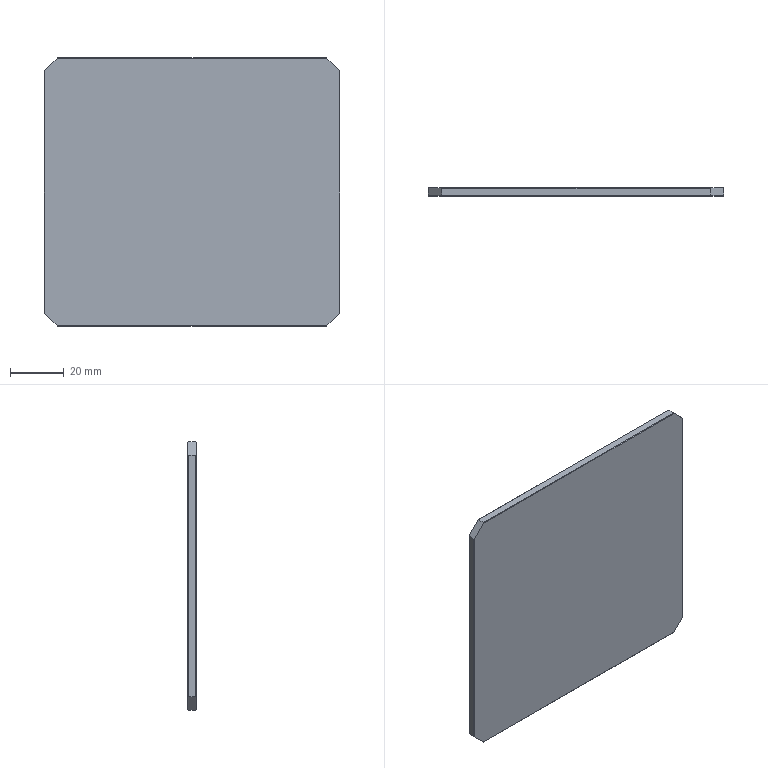Part | SolidWorks | features Chamfer 2, Extrusion 1, HoleWzd 1 | 1 solid | 18 faces | box 110 x 3 x 100 mm | volume 32835 mm3 | plane 18
STEP:
#1=CARTESIAN_POINT('',(-55.,2.8,-45.));
#2=VERTEX_POINT('',#1);
#3=CARTESIAN_POINT('',(-55.,0.2,-45.));
#4=VERTEX_POINT('',#3);
#5=CARTESIAN_POINT('',(-55.,3.,-45.));
#6=DIRECTION('',(0.,-1.,0.));
#7=VECTOR('',#6,1000.);
#8=LINE('',#5,#7);
#9=EDGE_CURVE('',#2,#4,#8,.T.);
#10=ORIENTED_EDGE('',*,*,#9,.T.);
#11=CARTESIAN_POINT('',(-55.,0.2,45.));
#12=VERTEX_POINT('',#11);
#13=CARTESIAN_POINT('',(-55.,0.2,50.));
#14=DIRECTION('',(0.,0.,1.));
#15=VECTOR('',#14,1000.);
#16=LINE('',#13,#15);
#17=EDGE_CURVE('',#4,#12,#16,.T.);
#18=ORIENTED_EDGE('',*,*,#17,.T.);
#19=CARTESIAN_POINT('',(-55.,2.8,45.));
#20=VERTEX_POINT('',#19);
#21=CARTESIAN_POINT('',(-55.,3.,45.));
#22=DIRECTION('',(0.,1.,0.));
#23=VECTOR('',#22,1000.);
#24=LINE('',#21,#23);
#25=EDGE_CURVE('',#12,#20,#24,.T.);
#26=ORIENTED_EDGE('',*,*,#25,.T.);
#27=CARTESIAN_POINT('',(-55.,2.8,-45.));
#28=DIRECTION('',(0.,0.,-1.));
#29=VECTOR('',#28,1000.);
#30=LINE('',#27,#29);
#31=EDGE_CURVE('',#20,#2,#30,.T.);
#32=ORIENTED_EDGE('',*,*,#31,.T.);
#33=EDGE_LOOP('',(#10,#18,#26,#32));
#34=FACE_OUTER_BOUND('',#33,.T.);
#35=CARTESIAN_POINT('',(-55.,3.,50.));
#36=DIRECTION('',(1.,0.,0.));
#37=DIRECTION('',(0.,0.,-1.));
#38=AXIS2_PLACEMENT_3D('',#35,#36,#37);
#39=PLANE('',#38);
#40=ADVANCED_FACE('',(#34),#39,.F.);
#41=CARTESIAN_POINT('',(-50.,2.8,50.));
#42=VERTEX_POINT('',#41);
#43=CARTESIAN_POINT('',(-50.,0.2,50.));
#44=VERTEX_POINT('',#43);
#45=CARTESIAN_POINT('',(-50.,3.,50.));
#46=DIRECTION('',(0.,-1.,0.));
#47=VECTOR('',#46,1000.);
#48=LINE('',#45,#47);
#49=EDGE_CURVE('',#42,#44,#48,.T.);
#50=ORIENTED_EDGE('',*,*,#49,.T.);
#51=CARTESIAN_POINT('',(50.,0.2,50.));
#52=VERTEX_POINT('',#51);
#53=CARTESIAN_POINT('',(55.,0.2,50.));
#54=DIRECTION('',(1.,0.,0.));
#55=VECTOR('',#54,1000.);
#56=LINE('',#53,#55);
#57=EDGE_CURVE('',#44,#52,#56,.T.);
#58=ORIENTED_EDGE('',*,*,#57,.T.);
#59=CARTESIAN_POINT('',(50.,2.8,50.));
#60=VERTEX_POINT('',#59);
#61=CARTESIAN_POINT('',(50.,3.,50.));
#62=DIRECTION('',(0.,1.,0.));
#63=VECTOR('',#62,1000.);
#64=LINE('',#61,#63);
#65=EDGE_CURVE('',#52,#60,#64,.T.);
#66=ORIENTED_EDGE('',*,*,#65,.T.);
#67=CARTESIAN_POINT('',(-50.,2.8,50.));
#68=DIRECTION('',(-1.,0.,0.));
#69=VECTOR('',#68,1000.);
#70=LINE('',#67,#69);
#71=EDGE_CURVE('',#60,#42,#70,.T.);
#72=ORIENTED_EDGE('',*,*,#71,.T.);
#73=EDGE_LOOP('',(#50,#58,#66,#72));
#74=FACE_OUTER_BOUND('',#73,.T.);
#75=CARTESIAN_POINT('',(55.,3.,50.));
#76=DIRECTION('',(0.,0.,-1.));
#77=DIRECTION('',(-1.,0.,0.));
#78=AXIS2_PLACEMENT_3D('',#75,#76,#77);
#79=PLANE('',#78);
#80=ADVANCED_FACE('',(#74),#79,.F.);
#81=CARTESIAN_POINT('',(55.,2.8,45.));
#82=VERTEX_POINT('',#81);
#83=CARTESIAN_POINT('',(55.,0.2,45.));
#84=VERTEX_POINT('',#83);
#85=CARTESIAN_POINT('',(55.,3.,45.));
#86=DIRECTION('',(0.,-1.,0.));
#87=VECTOR('',#86,1000.);
#88=LINE('',#85,#87);
#89=EDGE_CURVE('',#82,#84,#88,.T.);
#90=ORIENTED_EDGE('',*,*,#89,.T.);
#91=CARTESIAN_POINT('',(55.,0.2,-45.));
#92=VERTEX_POINT('',#91);
#93=CARTESIAN_POINT('',(55.,0.2,50.));
#94=DIRECTION('',(0.,0.,-1.));
#95=VECTOR('',#94,1000.);
#96=LINE('',#93,#95);
#97=EDGE_CURVE('',#84,#92,#96,.T.);
#98=ORIENTED_EDGE('',*,*,#97,.T.);
#99=CARTESIAN_POINT('',(55.,2.8,-45.));
#100=VERTEX_POINT('',#99);
#101=CARTESIAN_POINT('',(55.,3.,-45.));
#102=DIRECTION('',(0.,1.,0.));
#103=VECTOR('',#102,1000.);
#104=LINE('',#101,#103);
#105=EDGE_CURVE('',#92,#100,#104,.T.);
#106=ORIENTED_EDGE('',*,*,#105,.T.);
#107=CARTESIAN_POINT('',(55.,2.8,45.));
#108=DIRECTION('',(0.,0.,1.));
#109=VECTOR('',#108,1000.);
#110=LINE('',#107,#109);
#111=EDGE_CURVE('',#100,#82,#110,.T.);
#112=ORIENTED_EDGE('',*,*,#111,.T.);
#113=EDGE_LOOP('',(#90,#98,#106,#112));
#114=FACE_OUTER_BOUND('',#113,.T.);
#115=CARTESIAN_POINT('',(55.,3.,50.));
#116=DIRECTION('',(-1.,0.,0.));
#117=DIRECTION('',(0.,0.,1.));
#118=AXIS2_PLACEMENT_3D('',#115,#116,#117);
#119=PLANE('',#118);
#120=ADVANCED_FACE('',(#114),#119,.F.);
#121=CARTESIAN_POINT('',(50.,2.8,-50.));
#122=VERTEX_POINT('',#121);
#123=CARTESIAN_POINT('',(50.,0.2,-50.));
#124=VERTEX_POINT('',#123);
#125=CARTESIAN_POINT('',(50.,3.,-50.));
#126=DIRECTION('',(0.,-1.,0.));
#127=VECTOR('',#126,1000.);
#128=LINE('',#125,#127);
#129=EDGE_CURVE('',#122,#124,#128,.T.);
#130=ORIENTED_EDGE('',*,*,#129,.T.);
#131=CARTESIAN_POINT('',(-50.,0.2,-50.));
#132=VERTEX_POINT('',#131);
#133=CARTESIAN_POINT('',(55.,0.2,-50.));
#134=DIRECTION('',(-1.,0.,0.));
#135=VECTOR('',#134,1000.);
#136=LINE('',#133,#135);
#137=EDGE_CURVE('',#124,#132,#136,.T.);
#138=ORIENTED_EDGE('',*,*,#137,.T.);
#139=CARTESIAN_POINT('',(-50.,2.8,-50.));
#140=VERTEX_POINT('',#139);
#141=CARTESIAN_POINT('',(-50.,3.,-50.));
#142=DIRECTION('',(0.,1.,0.));
#143=VECTOR('',#142,1000.);
#144=LINE('',#141,#143);
#145=EDGE_CURVE('',#132,#140,#144,.T.);
#146=ORIENTED_EDGE('',*,*,#145,.T.);
#147=CARTESIAN_POINT('',(50.,2.8,-50.));
#148=DIRECTION('',(1.,0.,0.));
#149=VECTOR('',#148,1000.);
#150=LINE('',#147,#149);
#151=EDGE_CURVE('',#140,#122,#150,.T.);
#152=ORIENTED_EDGE('',*,*,#151,.T.);
#153=EDGE_LOOP('',(#130,#138,#146,#152));
#154=FACE_OUTER_BOUND('',#153,.T.);
#155=CARTESIAN_POINT('',(55.,3.,-50.));
#156=DIRECTION('',(0.,0.,1.));
#157=DIRECTION('',(1.,0.,0.));
#158=AXIS2_PLACEMENT_3D('',#155,#156,#157);
#159=PLANE('',#158);
#160=ADVANCED_FACE('',(#154),#159,.F.);
#161=CARTESIAN_POINT('',(50.2,3.,49.8));
#162=VERTEX_POINT('',#161);
#163=CARTESIAN_POINT('',(54.8,3.,45.2));
#164=VERTEX_POINT('',#163);
#165=CARTESIAN_POINT('',(50.,3.,50.));
#166=DIRECTION('',(0.7071,0.,-0.7071));
#167=VECTOR('',#166,1000.);
#168=LINE('',#165,#167);
#169=EDGE_CURVE('',#162,#164,#168,.T.);
#170=ORIENTED_EDGE('',*,*,#169,.T.);
#171=CARTESIAN_POINT('',(54.8,3.,-45.2));
#172=VERTEX_POINT('',#171);
#173=CARTESIAN_POINT('',(54.8,3.,-45.));
#174=DIRECTION('',(0.,0.,-1.));
#175=VECTOR('',#174,1000.);
#176=LINE('',#173,#175);
#177=EDGE_CURVE('',#164,#172,#176,.T.);
#178=ORIENTED_EDGE('',*,*,#177,.T.);
#179=CARTESIAN_POINT('',(50.2,3.,-49.8));
#180=VERTEX_POINT('',#179);
#181=CARTESIAN_POINT('',(50.,3.,-50.));
#182=DIRECTION('',(-0.7071,0.,-0.7071));
#183=VECTOR('',#182,1000.);
#184=LINE('',#181,#183);
#185=EDGE_CURVE('',#172,#180,#184,.T.);
#186=ORIENTED_EDGE('',*,*,#185,.T.);
#187=CARTESIAN_POINT('',(-50.2,3.,-49.8));
#188=VERTEX_POINT('',#187);
#189=CARTESIAN_POINT('',(-50.,3.,-49.8));
#190=DIRECTION('',(-1.,0.,0.));
#191=VECTOR('',#190,1000.);
#192=LINE('',#189,#191);
#193=EDGE_CURVE('',#180,#188,#192,.T.);
#194=ORIENTED_EDGE('',*,*,#193,.T.);
#195=CARTESIAN_POINT('',(-54.8,3.,-45.2));
#196=VERTEX_POINT('',#195);
#197=CARTESIAN_POINT('',(-50.,3.,-50.));
#198=DIRECTION('',(-0.7071,0.,0.7071));
#199=VECTOR('',#198,1000.);
#200=LINE('',#197,#199);
#201=EDGE_CURVE('',#188,#196,#200,.T.);
#202=ORIENTED_EDGE('',*,*,#201,.T.);
#203=CARTESIAN_POINT('',(-54.8,3.,45.2));
#204=VERTEX_POINT('',#203);
#205=CARTESIAN_POINT('',(-54.8,3.,45.));
#206=DIRECTION('',(0.,0.,1.));
#207=VECTOR('',#206,1000.);
#208=LINE('',#205,#207);
#209=EDGE_CURVE('',#196,#204,#208,.T.);
#210=ORIENTED_EDGE('',*,*,#209,.T.);
#211=CARTESIAN_POINT('',(-50.2,3.,49.8));
#212=VERTEX_POINT('',#211);
#213=CARTESIAN_POINT('',(-50.,3.,50.));
#214=DIRECTION('',(0.7071,0.,0.7071));
#215=VECTOR('',#214,1000.);
#216=LINE('',#213,#215);
#217=EDGE_CURVE('',#204,#212,#216,.T.);
#218=ORIENTED_EDGE('',*,*,#217,.T.);
#219=CARTESIAN_POINT('',(50.,3.,49.8));
#220=DIRECTION('',(1.,0.,0.));
#221=VECTOR('',#220,1000.);
#222=LINE('',#219,#221);
#223=EDGE_CURVE('',#212,#162,#222,.T.);
#224=ORIENTED_EDGE('',*,*,#223,.T.);
#225=EDGE_LOOP('',(#170,#178,#186,#194,#202,#210,#218,#224));
#226=FACE_OUTER_BOUND('',#225,.T.);
#227=CARTESIAN_POINT('',(0.,3.,0.));
#228=DIRECTION('',(0.,1.,0.));
#229=DIRECTION('',(0.,0.,1.));
#230=AXIS2_PLACEMENT_3D('',#227,#228,#229);
#231=PLANE('',#230);
#232=ADVANCED_FACE('',(#226),#231,.T.);
#233=CARTESIAN_POINT('',(-50.2,0.,49.8));
#234=VERTEX_POINT('',#233);
#235=CARTESIAN_POINT('',(-54.8,0.,45.2));
#236=VERTEX_POINT('',#235);
#237=CARTESIAN_POINT('',(-50.,0.,50.));
#238=DIRECTION('',(-0.7071,0.,-0.7071));
#239=VECTOR('',#238,1000.);
#240=LINE('',#237,#239);
#241=EDGE_CURVE('',#234,#236,#240,.T.);
#242=ORIENTED_EDGE('',*,*,#241,.T.);
#243=CARTESIAN_POINT('',(-54.8,0.,-45.2));
#244=VERTEX_POINT('',#243);
#245=CARTESIAN_POINT('',(-54.8,0.,0.));
#246=DIRECTION('',(0.,0.,-1.));
#247=VECTOR('',#246,1000.);
#248=LINE('',#245,#247);
#249=EDGE_CURVE('',#236,#244,#248,.T.);
#250=ORIENTED_EDGE('',*,*,#249,.T.);
#251=CARTESIAN_POINT('',(-50.2,0.,-49.8));
#252=VERTEX_POINT('',#251);
#253=CARTESIAN_POINT('',(-55.,0.,-45.));
#254=DIRECTION('',(0.7071,0.,-0.7071));
#255=VECTOR('',#254,1000.);
#256=LINE('',#253,#255);
#257=EDGE_CURVE('',#244,#252,#256,.T.);
#258=ORIENTED_EDGE('',*,*,#257,.T.);
#259=CARTESIAN_POINT('',(50.2,0.,-49.8));
#260=VERTEX_POINT('',#259);
#261=CARTESIAN_POINT('',(0.,0.,-49.8));
#262=DIRECTION('',(1.,0.,0.));
#263=VECTOR('',#262,1000.);
#264=LINE('',#261,#263);
#265=EDGE_CURVE('',#252,#260,#264,.T.);
#266=ORIENTED_EDGE('',*,*,#265,.T.);
#267=CARTESIAN_POINT('',(54.8,0.,-45.2));
#268=VERTEX_POINT('',#267);
#269=CARTESIAN_POINT('',(50.,0.,-50.));
#270=DIRECTION('',(0.7071,0.,0.7071));
#271=VECTOR('',#270,1000.);
#272=LINE('',#269,#271);
#273=EDGE_CURVE('',#260,#268,#272,.T.);
#274=ORIENTED_EDGE('',*,*,#273,.T.);
#275=CARTESIAN_POINT('',(54.8,0.,45.2));
#276=VERTEX_POINT('',#275);
#277=CARTESIAN_POINT('',(54.8,0.,0.));
#278=DIRECTION('',(0.,0.,1.));
#279=VECTOR('',#278,1000.);
#280=LINE('',#277,#279);
#281=EDGE_CURVE('',#268,#276,#280,.T.);
#282=ORIENTED_EDGE('',*,*,#281,.T.);
#283=CARTESIAN_POINT('',(50.2,0.,49.8));
#284=VERTEX_POINT('',#283);
#285=CARTESIAN_POINT('',(55.,0.,45.));
#286=DIRECTION('',(-0.7071,0.,0.7071));
#287=VECTOR('',#286,1000.);
#288=LINE('',#285,#287);
#289=EDGE_CURVE('',#276,#284,#288,.T.);
#290=ORIENTED_EDGE('',*,*,#289,.T.);
#291=CARTESIAN_POINT('',(0.,0.,49.8));
#292=DIRECTION('',(-1.,0.,0.));
#293=VECTOR('',#292,1000.);
#294=LINE('',#291,#293);
#295=EDGE_CURVE('',#284,#234,#294,.T.);
#296=ORIENTED_EDGE('',*,*,#295,.T.);
#297=EDGE_LOOP('',(#242,#250,#258,#266,#274,#282,#290,#296));
#298=FACE_OUTER_BOUND('',#297,.T.);
#299=CARTESIAN_POINT('',(0.,0.,0.));
#300=DIRECTION('',(0.,1.,0.));
#301=DIRECTION('',(0.,0.,1.));
#302=AXIS2_PLACEMENT_3D('',#299,#300,#301);
#303=PLANE('',#302);
#304=ADVANCED_FACE('',(#298),#303,.F.);
#305=ORIENTED_EDGE('',*,*,#25,.F.);
#306=CARTESIAN_POINT('',(-52.6,-2.2,47.4));
#307=DIRECTION('',(0.5774,-0.5774,0.5774));
#308=VECTOR('',#307,1000.);
#309=LINE('',#306,#308);
#310=EDGE_CURVE('',#12,#236,#309,.T.);
#311=ORIENTED_EDGE('',*,*,#310,.T.);
#312=ORIENTED_EDGE('',*,*,#241,.F.);
#313=CARTESIAN_POINT('',(-49.067,1.133,50.933));
#314=DIRECTION('',(0.5774,0.5774,0.5774));
#315=VECTOR('',#314,1000.);
#316=LINE('',#313,#315);
#317=EDGE_CURVE('',#234,#44,#316,.T.);
#318=ORIENTED_EDGE('',*,*,#317,.T.);
#319=ORIENTED_EDGE('',*,*,#49,.F.);
#320=CARTESIAN_POINT('',(-50.067,2.867,49.933));
#321=DIRECTION('',(-0.5774,0.5774,-0.5774));
#322=VECTOR('',#321,1000.);
#323=LINE('',#320,#322);
#324=EDGE_CURVE('',#42,#212,#323,.T.);
#325=ORIENTED_EDGE('',*,*,#324,.T.);
#326=ORIENTED_EDGE('',*,*,#217,.F.);
#327=CARTESIAN_POINT('',(-51.6,6.2,48.4));
#328=DIRECTION('',(-0.5774,-0.5774,-0.5774));
#329=VECTOR('',#328,1000.);
#330=LINE('',#327,#329);
#331=EDGE_CURVE('',#204,#20,#330,.T.);
#332=ORIENTED_EDGE('',*,*,#331,.T.);
#333=EDGE_LOOP('',(#305,#311,#312,#318,#319,#325,#326,#332));
#334=FACE_OUTER_BOUND('',#333,.T.);
#335=CARTESIAN_POINT('',(-50.,3.,50.));
#336=DIRECTION('',(0.7071,0.,-0.7071));
#337=DIRECTION('',(0.,-1.,0.));
#338=AXIS2_PLACEMENT_3D('',#335,#336,#337);
#339=PLANE('',#338);
#340=ADVANCED_FACE('',(#334),#339,.F.);
#341=ORIENTED_EDGE('',*,*,#257,.F.);
#342=CARTESIAN_POINT('',(-55.933,1.133,-44.067));
#343=DIRECTION('',(-0.5774,0.5774,0.5774));
#344=VECTOR('',#343,1000.);
#345=LINE('',#342,#344);
#346=EDGE_CURVE('',#244,#4,#345,.T.);
#347=ORIENTED_EDGE('',*,*,#346,.T.);
#348=ORIENTED_EDGE('',*,*,#9,.F.);
#349=CARTESIAN_POINT('',(-54.933,2.867,-45.067));
#350=DIRECTION('',(0.5774,0.5774,-0.5774));
#351=VECTOR('',#350,1000.);
#352=LINE('',#349,#351);
#353=EDGE_CURVE('',#2,#196,#352,.T.);
#354=ORIENTED_EDGE('',*,*,#353,.T.);
#355=ORIENTED_EDGE('',*,*,#201,.F.);
#356=CARTESIAN_POINT('',(-53.4,6.2,-46.6));
#357=DIRECTION('',(0.5774,-0.5774,-0.5774));
#358=VECTOR('',#357,1000.);
#359=LINE('',#356,#358);
#360=EDGE_CURVE('',#188,#140,#359,.T.);
#361=ORIENTED_EDGE('',*,*,#360,.T.);
#362=ORIENTED_EDGE('',*,*,#145,.F.);
#363=CARTESIAN_POINT('',(-52.4,-2.2,-47.6));
#364=DIRECTION('',(-0.5774,-0.5774,0.5774));
#365=VECTOR('',#364,1000.);
#366=LINE('',#363,#365);
#367=EDGE_CURVE('',#132,#252,#366,.T.);
#368=ORIENTED_EDGE('',*,*,#367,.T.);
#369=EDGE_LOOP('',(#341,#347,#348,#354,#355,#361,#362,#368));
#370=FACE_OUTER_BOUND('',#369,.T.);
#371=CARTESIAN_POINT('',(-55.,3.,-45.));
#372=DIRECTION('',(0.7071,0.,0.7071));
#373=DIRECTION('',(0.,-1.,0.));
#374=AXIS2_PLACEMENT_3D('',#371,#372,#373);
#375=PLANE('',#374);
#376=ADVANCED_FACE('',(#370),#375,.F.);
#377=ORIENTED_EDGE('',*,*,#273,.F.);
#378=CARTESIAN_POINT('',(49.067,1.133,-50.933));
#379=DIRECTION('',(-0.5774,0.5774,-0.5774));
#380=VECTOR('',#379,1000.);
#381=LINE('',#378,#380);
#382=EDGE_CURVE('',#260,#124,#381,.T.);
#383=ORIENTED_EDGE('',*,*,#382,.T.);
#384=ORIENTED_EDGE('',*,*,#129,.F.);
#385=CARTESIAN_POINT('',(50.067,2.867,-49.933));
#386=DIRECTION('',(0.5774,0.5774,0.5774));
#387=VECTOR('',#386,1000.);
#388=LINE('',#385,#387);
#389=EDGE_CURVE('',#122,#180,#388,.T.);
#390=ORIENTED_EDGE('',*,*,#389,.T.);
#391=ORIENTED_EDGE('',*,*,#185,.F.);
#392=CARTESIAN_POINT('',(51.6,6.2,-48.4));
#393=DIRECTION('',(0.5774,-0.5774,0.5774));
#394=VECTOR('',#393,1000.);
#395=LINE('',#392,#394);
#396=EDGE_CURVE('',#172,#100,#395,.T.);
#397=ORIENTED_EDGE('',*,*,#396,.T.);
#398=ORIENTED_EDGE('',*,*,#105,.F.);
#399=CARTESIAN_POINT('',(52.6,-2.2,-47.4));
#400=DIRECTION('',(-0.5774,-0.5774,-0.5774));
#401=VECTOR('',#400,1000.);
#402=LINE('',#399,#401);
#403=EDGE_CURVE('',#92,#268,#402,.T.);
#404=ORIENTED_EDGE('',*,*,#403,.T.);
#405=EDGE_LOOP('',(#377,#383,#384,#390,#391,#397,#398,#404));
#406=FACE_OUTER_BOUND('',#405,.T.);
#407=CARTESIAN_POINT('',(50.,3.,-50.));
#408=DIRECTION('',(-0.7071,0.,0.7071));
#409=DIRECTION('',(0.,-1.,0.));
#410=AXIS2_PLACEMENT_3D('',#407,#408,#409);
#411=PLANE('',#410);
#412=ADVANCED_FACE('',(#406),#411,.F.);
#413=ORIENTED_EDGE('',*,*,#65,.F.);
#414=CARTESIAN_POINT('',(52.4,-2.2,47.6));
#415=DIRECTION('',(0.5774,-0.5774,-0.5774));
#416=VECTOR('',#415,1000.);
#417=LINE('',#414,#416);
#418=EDGE_CURVE('',#52,#284,#417,.T.);
#419=ORIENTED_EDGE('',*,*,#418,.T.);
#420=ORIENTED_EDGE('',*,*,#289,.F.);
#421=CARTESIAN_POINT('',(55.933,1.133,44.067));
#422=DIRECTION('',(0.5774,0.5774,-0.5774));
#423=VECTOR('',#422,1000.);
#424=LINE('',#421,#423);
#425=EDGE_CURVE('',#276,#84,#424,.T.);
#426=ORIENTED_EDGE('',*,*,#425,.T.);
#427=ORIENTED_EDGE('',*,*,#89,.F.);
#428=CARTESIAN_POINT('',(54.933,2.867,45.067));
#429=DIRECTION('',(-0.5774,0.5774,0.5774));
#430=VECTOR('',#429,1000.);
#431=LINE('',#428,#430);
#432=EDGE_CURVE('',#82,#164,#431,.T.);
#433=ORIENTED_EDGE('',*,*,#432,.T.);
#434=ORIENTED_EDGE('',*,*,#169,.F.);
#435=CARTESIAN_POINT('',(53.4,6.2,46.6));
#436=DIRECTION('',(-0.5774,-0.5774,0.5774));
#437=VECTOR('',#436,1000.);
#438=LINE('',#435,#437);
#439=EDGE_CURVE('',#162,#60,#438,.T.);
#440=ORIENTED_EDGE('',*,*,#439,.T.);
#441=EDGE_LOOP('',(#413,#419,#420,#426,#427,#433,#434,#440));
#442=FACE_OUTER_BOUND('',#441,.T.);
#443=CARTESIAN_POINT('',(55.,3.,45.));
#444=DIRECTION('',(-0.7071,0.,-0.7071));
#445=DIRECTION('',(0.,-1.,0.));
#446=AXIS2_PLACEMENT_3D('',#443,#444,#445);
#447=PLANE('',#446);
#448=ADVANCED_FACE('',(#442),#447,.F.);
#449=ORIENTED_EDGE('',*,*,#346,.F.);
#450=ORIENTED_EDGE('',*,*,#249,.F.);
#451=ORIENTED_EDGE('',*,*,#310,.F.);
#452=ORIENTED_EDGE('',*,*,#17,.F.);
#453=EDGE_LOOP('',(#449,#450,#451,#452));
#454=FACE_OUTER_BOUND('',#453,.T.);
#455=CARTESIAN_POINT('',(-55.,0.2,50.));
#456=DIRECTION('',(0.7071,0.7071,0.));
#457=DIRECTION('',(0.,0.,1.));
#458=AXIS2_PLACEMENT_3D('',#455,#456,#457);
#459=PLANE('',#458);
#460=ADVANCED_FACE('',(#454),#459,.F.);
#461=ORIENTED_EDGE('',*,*,#382,.F.);
#462=ORIENTED_EDGE('',*,*,#265,.F.);
#463=ORIENTED_EDGE('',*,*,#367,.F.);
#464=ORIENTED_EDGE('',*,*,#137,.F.);
#465=EDGE_LOOP('',(#461,#462,#463,#464));
#466=FACE_OUTER_BOUND('',#465,.T.);
#467=CARTESIAN_POINT('',(55.,0.2,-50.));
#468=DIRECTION('',(0.,0.7071,0.7071));
#469=DIRECTION('',(-1.,0.,0.));
#470=AXIS2_PLACEMENT_3D('',#467,#468,#469);
#471=PLANE('',#470);
#472=ADVANCED_FACE('',(#466),#471,.F.);
#473=ORIENTED_EDGE('',*,*,#317,.F.);
#474=ORIENTED_EDGE('',*,*,#295,.F.);
#475=ORIENTED_EDGE('',*,*,#418,.F.);
#476=ORIENTED_EDGE('',*,*,#57,.F.);
#477=EDGE_LOOP('',(#473,#474,#475,#476));
#478=FACE_OUTER_BOUND('',#477,.T.);
#479=CARTESIAN_POINT('',(55.,0.2,50.));
#480=DIRECTION('',(0.,0.7071,-0.7071));
#481=DIRECTION('',(1.,0.,0.));
#482=AXIS2_PLACEMENT_3D('',#479,#480,#481);
#483=PLANE('',#482);
#484=ADVANCED_FACE('',(#478),#483,.F.);
#485=ORIENTED_EDGE('',*,*,#425,.F.);
#486=ORIENTED_EDGE('',*,*,#281,.F.);
#487=ORIENTED_EDGE('',*,*,#403,.F.);
#488=ORIENTED_EDGE('',*,*,#97,.F.);
#489=EDGE_LOOP('',(#485,#486,#487,#488));
#490=FACE_OUTER_BOUND('',#489,.T.);
#491=CARTESIAN_POINT('',(55.,0.2,50.));
#492=DIRECTION('',(-0.7071,0.7071,0.));
#493=DIRECTION('',(0.,0.,-1.));
#494=AXIS2_PLACEMENT_3D('',#491,#492,#493);
#495=PLANE('',#494);
#496=ADVANCED_FACE('',(#490),#495,.F.);
#497=ORIENTED_EDGE('',*,*,#432,.F.);
#498=ORIENTED_EDGE('',*,*,#111,.F.);
#499=ORIENTED_EDGE('',*,*,#396,.F.);
#500=ORIENTED_EDGE('',*,*,#177,.F.);
#501=EDGE_LOOP('',(#497,#498,#499,#500));
#502=FACE_OUTER_BOUND('',#501,.T.);
#503=CARTESIAN_POINT('',(54.8,3.,0.));
#504=DIRECTION('',(0.7071,0.7071,0.));
#505=DIRECTION('',(0.,0.,1.));
#506=AXIS2_PLACEMENT_3D('',#503,#504,#505);
#507=PLANE('',#506);
#508=ADVANCED_FACE('',(#502),#507,.T.);
#509=ORIENTED_EDGE('',*,*,#389,.F.);
#510=ORIENTED_EDGE('',*,*,#151,.F.);
#511=ORIENTED_EDGE('',*,*,#360,.F.);
#512=ORIENTED_EDGE('',*,*,#193,.F.);
#513=EDGE_LOOP('',(#509,#510,#511,#512));
#514=FACE_OUTER_BOUND('',#513,.T.);
#515=CARTESIAN_POINT('',(0.,3.,-49.8));
#516=DIRECTION('',(0.,0.7071,-0.7071));
#517=DIRECTION('',(1.,0.,0.));
#518=AXIS2_PLACEMENT_3D('',#515,#516,#517);
#519=PLANE('',#518);
#520=ADVANCED_FACE('',(#514),#519,.T.);
#521=ORIENTED_EDGE('',*,*,#353,.F.);
#522=ORIENTED_EDGE('',*,*,#31,.F.);
#523=ORIENTED_EDGE('',*,*,#331,.F.);
#524=ORIENTED_EDGE('',*,*,#209,.F.);
#525=EDGE_LOOP('',(#521,#522,#523,#524));
#526=FACE_OUTER_BOUND('',#525,.T.);
#527=CARTESIAN_POINT('',(-54.8,3.,0.));
#528=DIRECTION('',(-0.7071,0.7071,0.));
#529=DIRECTION('',(0.,0.,-1.));
#530=AXIS2_PLACEMENT_3D('',#527,#528,#529);
#531=PLANE('',#530);
#532=ADVANCED_FACE('',(#526),#531,.T.);
#533=ORIENTED_EDGE('',*,*,#324,.F.);
#534=ORIENTED_EDGE('',*,*,#71,.F.);
#535=ORIENTED_EDGE('',*,*,#439,.F.);
#536=ORIENTED_EDGE('',*,*,#223,.F.);
#537=EDGE_LOOP('',(#533,#534,#535,#536));
#538=FACE_OUTER_BOUND('',#537,.T.);
#539=CARTESIAN_POINT('',(0.,3.,49.8));
#540=DIRECTION('',(0.,0.7071,0.7071));
#541=DIRECTION('',(-1.,0.,0.));
#542=AXIS2_PLACEMENT_3D('',#539,#540,#541);
#543=PLANE('',#542);
#544=ADVANCED_FACE('',(#538),#543,.T.);
#545=CLOSED_SHELL('',(#40,#80,#120,#160,#232,#304,#340,#376,#412,#448,#460,#472,#484,#496,#508,#520,#532,#544));
#546=MANIFOLD_SOLID_BREP('',#545);
#547=CARTESIAN_POINT('',(0.,0.,0.));
#548=DIRECTION('',(0.,0.,1.));
#549=DIRECTION('',(1.,0.,0.));
#550=AXIS2_PLACEMENT_3D('',#547,#548,#549);
#551=(LENGTH_UNIT()NAMED_UNIT(*)SI_UNIT(.MILLI.,.METRE.));
#552=UNCERTAINTY_MEASURE_WITH_UNIT(LENGTH_MEASURE(0.00001),#551,'','');
#553=(NAMED_UNIT(*)PLANE_ANGLE_UNIT()SI_UNIT($,.RADIAN.));
#554=(NAMED_UNIT(*)SI_UNIT($,.STERADIAN.)SOLID_ANGLE_UNIT());
#555=(GEOMETRIC_REPRESENTATION_CONTEXT(3)GLOBAL_UNCERTAINTY_ASSIGNED_CONTEXT((#552))GLOBAL_UNIT_ASSIGNED_CONTEXT((#551,#553,#554))REPRESENTATION_CONTEXT('',''));
#556=ADVANCED_BREP_SHAPE_REPRESENTATION('',(#546,#550),#555);